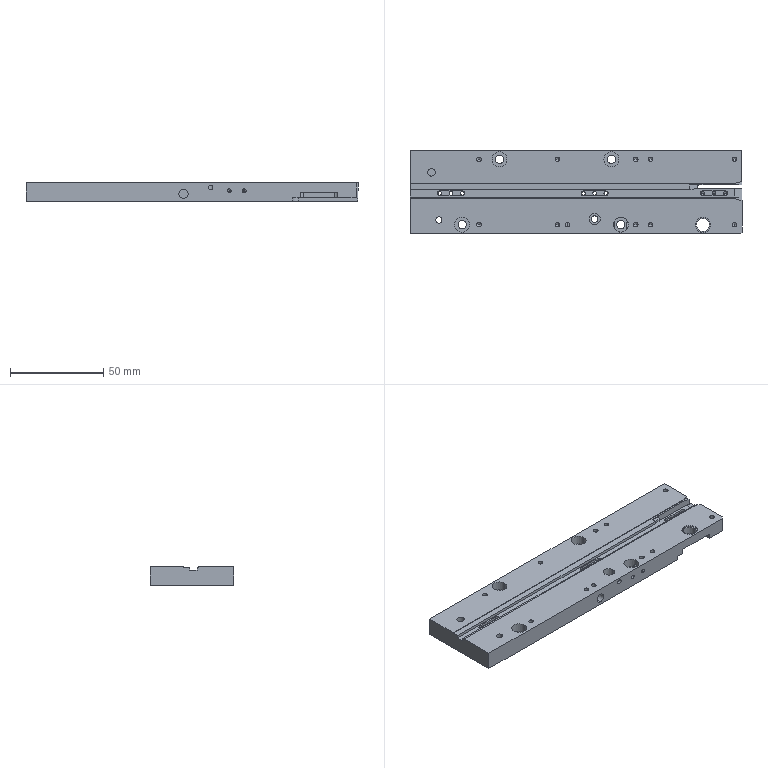Part | SolidWorks | features ICE 30, HoleWzd 8, Chamfer 7, Fillet 6, 3DProfileFeature 4, Cut 4, Extrusion 1 | 1 solid | 203 faces | box 178 x 45 x 10 mm | volume 72367 mm3 | cylinder 109 | plane 68 | cone 26 | commonest cylinder face diameters 2.5 x33 2 x23 4 x10 2.05 x8 4.5 x8 8 x8